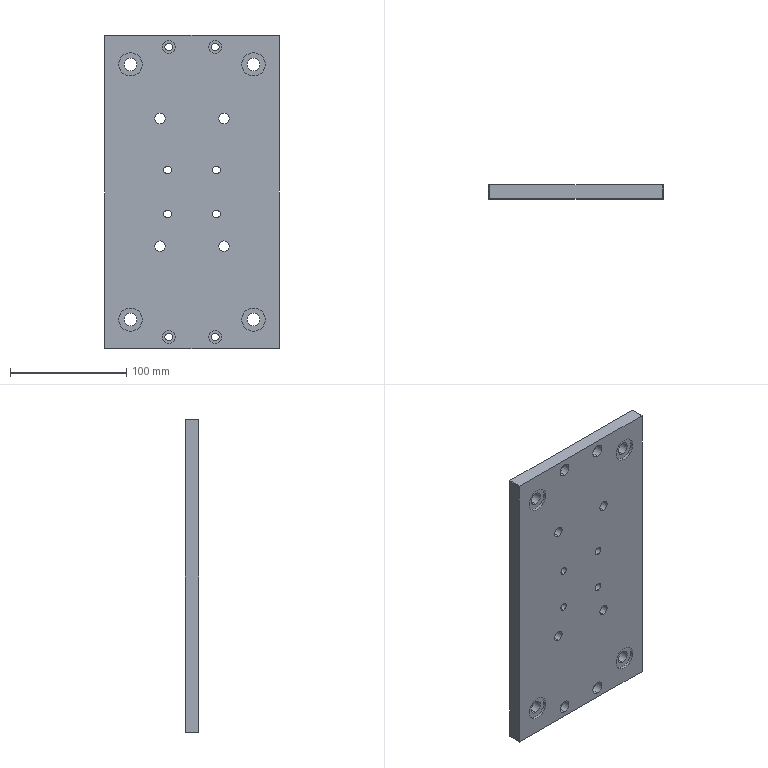Part | SolidWorks | features HoleWzd 5, ICE 2, Chamfer 1, Extrusion 1 | 1 solid | 78 faces | box 150 x 12 x 270 mm | volume 470446 mm3 | cylinder 56 | plane 22 | commonest cylinder face diameters 11 x16 6.6 x8 6.8 x8 9 x8 15 x8 20 x8